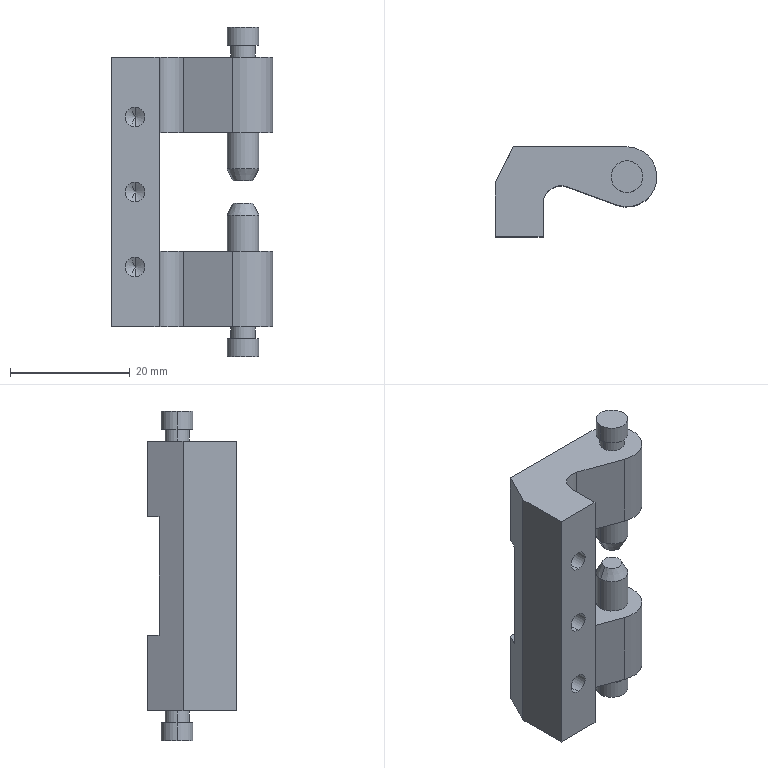Part | SolidWorks | features BaseBody 1 | 1 solid | 51 faces | box 27 x 15 x 55 mm | volume 8868 mm3 | cylinder 22 | plane 19 | cone 10 | commonest cylinder face diameters 5.3 x8 3.3 x6 4.101 x4 6 x2 10 x2
STEP:
#1=CARTESIAN_POINT('',(4.,13.,-9.85));
#2=VERTEX_POINT('',#1);
#3=CARTESIAN_POINT('',(-2.,13.,-9.85));
#4=VERTEX_POINT('',#3);
#5=CARTESIAN_POINT('',(11.,13.,-9.85));
#6=DIRECTION('',(-1.,0.,0.));
#7=VECTOR('',#6,1000.);
#8=LINE('',#5,#7);
#9=EDGE_CURVE('',#2,#4,#8,.T.);
#10=ORIENTED_EDGE('',*,*,#9,.T.);
#11=CARTESIAN_POINT('',(-2.,13.,9.85));
#12=VERTEX_POINT('',#11);
#13=CARTESIAN_POINT('',(-2.,13.,22.5));
#14=DIRECTION('',(0.,0.,-1.));
#15=VECTOR('',#14,1000.);
#16=LINE('',#13,#15);
#17=EDGE_CURVE('',#12,#4,#16,.T.);
#18=ORIENTED_EDGE('',*,*,#17,.F.);
#19=CARTESIAN_POINT('',(4.,13.,9.85));
#20=VERTEX_POINT('',#19);
#21=CARTESIAN_POINT('',(11.,13.,9.85));
#22=DIRECTION('',(-1.,0.,0.));
#23=VECTOR('',#22,1000.);
#24=LINE('',#21,#23);
#25=EDGE_CURVE('',#20,#12,#24,.T.);
#26=ORIENTED_EDGE('',*,*,#25,.F.);
#27=CARTESIAN_POINT('',(4.,13.,22.5));
#28=DIRECTION('',(0.,0.,1.));
#29=VECTOR('',#28,1000.);
#30=LINE('',#27,#29);
#31=EDGE_CURVE('',#2,#20,#30,.T.);
#32=ORIENTED_EDGE('',*,*,#31,.F.);
#33=EDGE_LOOP('',(#10,#18,#26,#32));
#34=FACE_OUTER_BOUND('',#33,.T.);
#35=CARTESIAN_POINT('',(11.,13.,-9.85));
#36=DIRECTION('',(0.,-1.,0.));
#37=DIRECTION('',(0.,0.,-1.));
#38=AXIS2_PLACEMENT_3D('',#35,#36,#37);
#39=PLANE('',#38);
#40=ADVANCED_FACE('',(#34),#39,.F.);
#41=CARTESIAN_POINT('',(0.,10.1,1.65));
#42=VERTEX_POINT('',#41);
#43=CARTESIAN_POINT('',(0.,0.,1.65));
#44=VERTEX_POINT('',#43);
#45=CARTESIAN_POINT('',(0.,0.,1.65));
#46=DIRECTION('',(0.,-1.,0.));
#47=VECTOR('',#46,1000.);
#48=LINE('',#45,#47);
#49=EDGE_CURVE('',#42,#44,#48,.T.);
#50=ORIENTED_EDGE('',*,*,#49,.F.);
#51=CARTESIAN_POINT('',(0.,10.1,-1.65));
#52=VERTEX_POINT('',#51);
#53=CARTESIAN_POINT('',(0.,10.1,0.));
#54=DIRECTION('',(0.,-1.,0.));
#55=DIRECTION('',(0.,0.,-1.));
#56=AXIS2_PLACEMENT_3D('',#53,#54,#55);
#57=CIRCLE('',#56,1.65);
#58=EDGE_CURVE('',#52,#42,#57,.T.);
#59=ORIENTED_EDGE('',*,*,#58,.F.);
#60=CARTESIAN_POINT('',(0.,0.,-1.65));
#61=VERTEX_POINT('',#60);
#62=CARTESIAN_POINT('',(0.,0.,-1.65));
#63=DIRECTION('',(0.,-1.,0.));
#64=VECTOR('',#63,1000.);
#65=LINE('',#62,#64);
#66=EDGE_CURVE('',#52,#61,#65,.T.);
#67=ORIENTED_EDGE('',*,*,#66,.T.);
#68=CARTESIAN_POINT('',(0.,0.,0.));
#69=DIRECTION('',(0.,-1.,0.));
#70=DIRECTION('',(0.,0.,-1.));
#71=AXIS2_PLACEMENT_3D('',#68,#69,#70);
#72=CIRCLE('',#71,1.65);
#73=EDGE_CURVE('',#61,#44,#72,.T.);
#74=ORIENTED_EDGE('',*,*,#73,.T.);
#75=EDGE_LOOP('',(#50,#59,#67,#74));
#76=FACE_OUTER_BOUND('',#75,.T.);
#77=CARTESIAN_POINT('',(0.,0.,0.));
#78=DIRECTION('',(0.,-1.,0.));
#79=DIRECTION('',(0.,0.,-1.));
#80=AXIS2_PLACEMENT_3D('',#77,#78,#79);
#81=CYLINDRICAL_SURFACE('',#80,1.65);
#82=ADVANCED_FACE('',(#76),#81,.F.);
#83=CARTESIAN_POINT('',(0.,11.091,0.));
#84=VERTEX_POINT('',#83);
#85=CARTESIAN_POINT('',(0.,10.1,1.65));
#86=DIRECTION('',(0.,-0.515,0.8572));
#87=VECTOR('',#86,1000.);
#88=LINE('',#85,#87);
#89=EDGE_CURVE('',#84,#42,#88,.T.);
#90=ORIENTED_EDGE('',*,*,#89,.F.);
#91=CARTESIAN_POINT('',(0.,10.1,-1.65));
#92=DIRECTION('',(0.,-0.515,-0.8572));
#93=VECTOR('',#92,1000.);
#94=LINE('',#91,#93);
#95=EDGE_CURVE('',#84,#52,#94,.T.);
#96=ORIENTED_EDGE('',*,*,#95,.T.);
#97=ORIENTED_EDGE('',*,*,#58,.T.);
#98=EDGE_LOOP('',(#90,#96,#97));
#99=FACE_OUTER_BOUND('',#98,.T.);
#100=CARTESIAN_POINT('',(0.,10.1,0.));
#101=DIRECTION('',(0.,-1.,0.));
#102=DIRECTION('',(0.,0.,-1.));
#103=AXIS2_PLACEMENT_3D('',#100,#101,#102);
#104=CONICAL_SURFACE('',#103,1.65,1.03);
#105=ADVANCED_FACE('',(#99),#104,.F.);
#106=CARTESIAN_POINT('',(0.,10.1,14.15));
#107=VERTEX_POINT('',#106);
#108=CARTESIAN_POINT('',(0.,0.,14.15));
#109=VERTEX_POINT('',#108);
#110=CARTESIAN_POINT('',(0.,0.,14.15));
#111=DIRECTION('',(0.,-1.,0.));
#112=VECTOR('',#111,1000.);
#113=LINE('',#110,#112);
#114=EDGE_CURVE('',#107,#109,#113,.T.);
#115=ORIENTED_EDGE('',*,*,#114,.F.);
#116=CARTESIAN_POINT('',(0.,10.1,10.85));
#117=VERTEX_POINT('',#116);
#118=CARTESIAN_POINT('',(0.,10.1,12.5));
#119=DIRECTION('',(0.,-1.,0.));
#120=DIRECTION('',(0.,0.,-1.));
#121=AXIS2_PLACEMENT_3D('',#118,#119,#120);
#122=CIRCLE('',#121,1.65);
#123=EDGE_CURVE('',#117,#107,#122,.T.);
#124=ORIENTED_EDGE('',*,*,#123,.F.);
#125=CARTESIAN_POINT('',(0.,0.,10.85));
#126=VERTEX_POINT('',#125);
#127=CARTESIAN_POINT('',(0.,0.,10.85));
#128=DIRECTION('',(0.,-1.,0.));
#129=VECTOR('',#128,1000.);
#130=LINE('',#127,#129);
#131=EDGE_CURVE('',#117,#126,#130,.T.);
#132=ORIENTED_EDGE('',*,*,#131,.T.);
#133=CARTESIAN_POINT('',(0.,0.,12.5));
#134=DIRECTION('',(0.,-1.,0.));
#135=DIRECTION('',(0.,0.,-1.));
#136=AXIS2_PLACEMENT_3D('',#133,#134,#135);
#137=CIRCLE('',#136,1.65);
#138=EDGE_CURVE('',#126,#109,#137,.T.);
#139=ORIENTED_EDGE('',*,*,#138,.T.);
#140=EDGE_LOOP('',(#115,#124,#132,#139));
#141=FACE_OUTER_BOUND('',#140,.T.);
#142=CARTESIAN_POINT('',(0.,0.,12.5));
#143=DIRECTION('',(0.,-1.,0.));
#144=DIRECTION('',(0.,0.,-1.));
#145=AXIS2_PLACEMENT_3D('',#142,#143,#144);
#146=CYLINDRICAL_SURFACE('',#145,1.65);
#147=ADVANCED_FACE('',(#141),#146,.F.);
#148=CARTESIAN_POINT('',(0.,11.091,12.5));
#149=VERTEX_POINT('',#148);
#150=CARTESIAN_POINT('',(0.,10.1,14.15));
#151=DIRECTION('',(0.,-0.515,0.8572));
#152=VECTOR('',#151,1000.);
#153=LINE('',#150,#152);
#154=EDGE_CURVE('',#149,#107,#153,.T.);
#155=ORIENTED_EDGE('',*,*,#154,.F.);
#156=CARTESIAN_POINT('',(0.,10.1,10.85));
#157=DIRECTION('',(0.,-0.515,-0.8572));
#158=VECTOR('',#157,1000.);
#159=LINE('',#156,#158);
#160=EDGE_CURVE('',#149,#117,#159,.T.);
#161=ORIENTED_EDGE('',*,*,#160,.T.);
#162=ORIENTED_EDGE('',*,*,#123,.T.);
#163=EDGE_LOOP('',(#155,#161,#162));
#164=FACE_OUTER_BOUND('',#163,.T.);
#165=CARTESIAN_POINT('',(0.,10.1,12.5));
#166=DIRECTION('',(0.,-1.,0.));
#167=DIRECTION('',(0.,0.,-1.));
#168=AXIS2_PLACEMENT_3D('',#165,#166,#167);
#169=CONICAL_SURFACE('',#168,1.65,1.03);
#170=ADVANCED_FACE('',(#164),#169,.F.);
#171=CARTESIAN_POINT('',(0.,10.1,-10.85));
#172=VERTEX_POINT('',#171);
#173=CARTESIAN_POINT('',(0.,0.,-10.85));
#174=VERTEX_POINT('',#173);
#175=CARTESIAN_POINT('',(0.,0.,-10.85));
#176=DIRECTION('',(0.,-1.,0.));
#177=VECTOR('',#176,1000.);
#178=LINE('',#175,#177);
#179=EDGE_CURVE('',#172,#174,#178,.T.);
#180=ORIENTED_EDGE('',*,*,#179,.F.);
#181=CARTESIAN_POINT('',(0.,10.1,-14.15));
#182=VERTEX_POINT('',#181);
#183=CARTESIAN_POINT('',(0.,10.1,-12.5));
#184=DIRECTION('',(0.,-1.,0.));
#185=DIRECTION('',(0.,0.,-1.));
#186=AXIS2_PLACEMENT_3D('',#183,#184,#185);
#187=CIRCLE('',#186,1.65);
#188=EDGE_CURVE('',#182,#172,#187,.T.);
#189=ORIENTED_EDGE('',*,*,#188,.F.);
#190=CARTESIAN_POINT('',(0.,0.,-14.15));
#191=VERTEX_POINT('',#190);
#192=CARTESIAN_POINT('',(0.,0.,-14.15));
#193=DIRECTION('',(0.,-1.,0.));
#194=VECTOR('',#193,1000.);
#195=LINE('',#192,#194);
#196=EDGE_CURVE('',#182,#191,#195,.T.);
#197=ORIENTED_EDGE('',*,*,#196,.T.);
#198=CARTESIAN_POINT('',(0.,0.,-12.5));
#199=DIRECTION('',(0.,-1.,0.));
#200=DIRECTION('',(0.,0.,-1.));
#201=AXIS2_PLACEMENT_3D('',#198,#199,#200);
#202=CIRCLE('',#201,1.65);
#203=EDGE_CURVE('',#191,#174,#202,.T.);
#204=ORIENTED_EDGE('',*,*,#203,.T.);
#205=EDGE_LOOP('',(#180,#189,#197,#204));
#206=FACE_OUTER_BOUND('',#205,.T.);
#207=CARTESIAN_POINT('',(0.,0.,-12.5));
#208=DIRECTION('',(0.,-1.,0.));
#209=DIRECTION('',(0.,0.,-1.));
#210=AXIS2_PLACEMENT_3D('',#207,#208,#209);
#211=CYLINDRICAL_SURFACE('',#210,1.65);
#212=ADVANCED_FACE('',(#206),#211,.F.);
#213=CARTESIAN_POINT('',(0.,11.091,-12.5));
#214=VERTEX_POINT('',#213);
#215=CARTESIAN_POINT('',(0.,10.1,-10.85));
#216=DIRECTION('',(0.,-0.515,0.8572));
#217=VECTOR('',#216,1000.);
#218=LINE('',#215,#217);
#219=EDGE_CURVE('',#214,#172,#218,.T.);
#220=ORIENTED_EDGE('',*,*,#219,.F.);
#221=CARTESIAN_POINT('',(0.,10.1,-14.15));
#222=DIRECTION('',(0.,-0.515,-0.8572));
#223=VECTOR('',#222,1000.);
#224=LINE('',#221,#223);
#225=EDGE_CURVE('',#214,#182,#224,.T.);
#226=ORIENTED_EDGE('',*,*,#225,.T.);
#227=ORIENTED_EDGE('',*,*,#188,.T.);
#228=EDGE_LOOP('',(#220,#226,#227));
#229=FACE_OUTER_BOUND('',#228,.T.);
#230=CARTESIAN_POINT('',(0.,10.1,-12.5));
#231=DIRECTION('',(0.,-1.,0.));
#232=DIRECTION('',(0.,0.,-1.));
#233=AXIS2_PLACEMENT_3D('',#230,#231,#232);
#234=CONICAL_SURFACE('',#233,1.65,1.03);
#235=ADVANCED_FACE('',(#229),#234,.F.);
#236=CARTESIAN_POINT('',(20.65,10.,27.5));
#237=VERTEX_POINT('',#236);
#238=CARTESIAN_POINT('',(20.65,10.,24.5));
#239=VERTEX_POINT('',#238);
#240=CARTESIAN_POINT('',(20.65,10.,27.5));
#241=DIRECTION('',(0.,0.,-1.));
#242=VECTOR('',#241,1000.);
#243=LINE('',#240,#242);
#244=EDGE_CURVE('',#237,#239,#243,.T.);
#245=ORIENTED_EDGE('',*,*,#244,.F.);
#246=CARTESIAN_POINT('',(15.35,10.,27.5));
#247=VERTEX_POINT('',#246);
#248=CARTESIAN_POINT('',(18.,10.,27.5));
#249=DIRECTION('',(0.,0.,-1.));
#250=DIRECTION('',(-1.,0.,0.));
#251=AXIS2_PLACEMENT_3D('',#248,#249,#250);
#252=CIRCLE('',#251,2.65);
#253=EDGE_CURVE('',#237,#247,#252,.T.);
#254=ORIENTED_EDGE('',*,*,#253,.T.);
#255=CARTESIAN_POINT('',(15.35,10.,24.5));
#256=VERTEX_POINT('',#255);
#257=CARTESIAN_POINT('',(15.35,10.,27.5));
#258=DIRECTION('',(0.,0.,-1.));
#259=VECTOR('',#258,1000.);
#260=LINE('',#257,#259);
#261=EDGE_CURVE('',#247,#256,#260,.T.);
#262=ORIENTED_EDGE('',*,*,#261,.T.);
#263=CARTESIAN_POINT('',(18.,10.,24.5));
#264=DIRECTION('',(0.,0.,-1.));
#265=DIRECTION('',(-1.,0.,0.));
#266=AXIS2_PLACEMENT_3D('',#263,#264,#265);
#267=CIRCLE('',#266,2.65);
#268=EDGE_CURVE('',#239,#256,#267,.T.);
#269=ORIENTED_EDGE('',*,*,#268,.F.);
#270=EDGE_LOOP('',(#245,#254,#262,#269));
#271=FACE_OUTER_BOUND('',#270,.T.);
#272=CARTESIAN_POINT('',(18.,10.,27.5));
#273=DIRECTION('',(0.,0.,-1.));
#274=DIRECTION('',(-1.,0.,0.));
#275=AXIS2_PLACEMENT_3D('',#272,#273,#274);
#276=CYLINDRICAL_SURFACE('',#275,2.65);
#277=ADVANCED_FACE('',(#271),#276,.T.);
#278=CARTESIAN_POINT('',(18.,10.,27.5));
#279=DIRECTION('',(0.,0.,-1.));
#280=DIRECTION('',(-1.,0.,0.));
#281=AXIS2_PLACEMENT_3D('',#278,#279,#280);
#282=CIRCLE('',#281,2.65);
#283=EDGE_CURVE('',#247,#237,#282,.T.);
#284=ORIENTED_EDGE('',*,*,#283,.F.);
#285=ORIENTED_EDGE('',*,*,#253,.F.);
#286=EDGE_LOOP('',(#284,#285));
#287=FACE_OUTER_BOUND('',#286,.T.);
#288=CARTESIAN_POINT('',(18.,10.,27.5));
#289=DIRECTION('',(0.,0.,1.));
#290=DIRECTION('',(1.,0.,0.));
#291=AXIS2_PLACEMENT_3D('',#288,#289,#290);
#292=PLANE('',#291);
#293=ADVANCED_FACE('',(#287),#292,.T.);
#294=CARTESIAN_POINT('',(20.05,10.,24.5));
#295=VERTEX_POINT('',#294);
#296=CARTESIAN_POINT('',(20.05,10.,22.5));
#297=VERTEX_POINT('',#296);
#298=CARTESIAN_POINT('',(20.05,10.,24.5));
#299=DIRECTION('',(0.,0.,-1.));
#300=VECTOR('',#299,1000.);
#301=LINE('',#298,#300);
#302=EDGE_CURVE('',#295,#297,#301,.T.);
#303=ORIENTED_EDGE('',*,*,#302,.F.);
#304=CARTESIAN_POINT('',(15.95,10.,24.5));
#305=VERTEX_POINT('',#304);
#306=CARTESIAN_POINT('',(18.,10.,24.5));
#307=DIRECTION('',(0.,0.,-1.));
#308=DIRECTION('',(-1.,0.,0.));
#309=AXIS2_PLACEMENT_3D('',#306,#307,#308);
#310=CIRCLE('',#309,2.05);
#311=EDGE_CURVE('',#295,#305,#310,.T.);
#312=ORIENTED_EDGE('',*,*,#311,.T.);
#313=CARTESIAN_POINT('',(15.95,10.,22.5));
#314=VERTEX_POINT('',#313);
#315=CARTESIAN_POINT('',(15.95,10.,24.5));
#316=DIRECTION('',(0.,0.,-1.));
#317=VECTOR('',#316,1000.);
#318=LINE('',#315,#317);
#319=EDGE_CURVE('',#305,#314,#318,.T.);
#320=ORIENTED_EDGE('',*,*,#319,.T.);
#321=CARTESIAN_POINT('',(18.,10.,22.5));
#322=DIRECTION('',(0.,0.,-1.));
#323=DIRECTION('',(-1.,0.,0.));
#324=AXIS2_PLACEMENT_3D('',#321,#322,#323);
#325=CIRCLE('',#324,2.05);
#326=EDGE_CURVE('',#297,#314,#325,.T.);
#327=ORIENTED_EDGE('',*,*,#326,.F.);
#328=EDGE_LOOP('',(#303,#312,#320,#327));
#329=FACE_OUTER_BOUND('',#328,.T.);
#330=CARTESIAN_POINT('',(18.,10.,24.5));
#331=DIRECTION('',(0.,0.,-1.));
#332=DIRECTION('',(-1.,0.,0.));
#333=AXIS2_PLACEMENT_3D('',#330,#331,#332);
#334=CYLINDRICAL_SURFACE('',#333,2.05);
#335=ADVANCED_FACE('',(#329),#334,.T.);
#336=CARTESIAN_POINT('',(18.,10.,24.5));
#337=DIRECTION('',(0.,0.,-1.));
#338=DIRECTION('',(-1.,0.,0.));
#339=AXIS2_PLACEMENT_3D('',#336,#337,#338);
#340=CIRCLE('',#339,2.05);
#341=EDGE_CURVE('',#305,#295,#340,.T.);
#342=ORIENTED_EDGE('',*,*,#341,.F.);
#343=ORIENTED_EDGE('',*,*,#311,.F.);
#344=EDGE_LOOP('',(#342,#343));
#345=FACE_BOUND('',#344,.T.);
#346=CARTESIAN_POINT('',(18.,10.,24.5));
#347=DIRECTION('',(0.,0.,-1.));
#348=DIRECTION('',(-1.,0.,0.));
#349=AXIS2_PLACEMENT_3D('',#346,#347,#348);
#350=CIRCLE('',#349,2.65);
#351=EDGE_CURVE('',#256,#239,#350,.T.);
#352=ORIENTED_EDGE('',*,*,#351,.T.);
#353=ORIENTED_EDGE('',*,*,#268,.T.);
#354=EDGE_LOOP('',(#352,#353));
#355=FACE_OUTER_BOUND('',#354,.T.);
#356=CARTESIAN_POINT('',(18.,10.,24.5));
#357=DIRECTION('',(0.,0.,1.));
#358=DIRECTION('',(1.,0.,0.));
#359=AXIS2_PLACEMENT_3D('',#356,#357,#358);
#360=PLANE('',#359);
#361=ADVANCED_FACE('',(#345,#355),#360,.F.);
#362=CARTESIAN_POINT('',(16.35,10.,1.85));
#363=VERTEX_POINT('',#362);
#364=CARTESIAN_POINT('',(15.35,10.,3.85));
#365=VERTEX_POINT('',#364);
#366=CARTESIAN_POINT('',(15.35,10.,3.85));
#367=DIRECTION('',(-0.4472,0.,0.8944));
#368=VECTOR('',#367,1000.);
#369=LINE('',#366,#368);
#370=EDGE_CURVE('',#363,#365,#369,.T.);
#371=ORIENTED_EDGE('',*,*,#370,.F.);
#372=CARTESIAN_POINT('',(19.65,10.,1.85));
#373=VERTEX_POINT('',#372);
#374=CARTESIAN_POINT('',(18.,10.,1.85));
#375=DIRECTION('',(0.,0.,-1.));
#376=DIRECTION('',(-1.,0.,0.));
#377=AXIS2_PLACEMENT_3D('',#374,#375,#376);
#378=CIRCLE('',#377,1.65);
#379=EDGE_CURVE('',#373,#363,#378,.T.);
#380=ORIENTED_EDGE('',*,*,#379,.F.);
#381=CARTESIAN_POINT('',(20.65,10.,3.85));
#382=VERTEX_POINT('',#381);
#383=CARTESIAN_POINT('',(20.65,10.,3.85));
#384=DIRECTION('',(0.4472,0.,0.8944));
#385=VECTOR('',#384,1000.);
#386=LINE('',#383,#385);
#387=EDGE_CURVE('',#373,#382,#386,.T.);
#388=ORIENTED_EDGE('',*,*,#387,.T.);
#389=CARTESIAN_POINT('',(18.,10.,3.85));
#390=DIRECTION('',(0.,0.,1.));
#391=DIRECTION('',(-1.,0.,0.));
#392=AXIS2_PLACEMENT_3D('',#389,#390,#391);
#393=CIRCLE('',#392,2.65);
#394=EDGE_CURVE('',#365,#382,#393,.T.);
#395=ORIENTED_EDGE('',*,*,#394,.F.);
#396=EDGE_LOOP('',(#371,#380,#388,#395));
#397=FACE_OUTER_BOUND('',#396,.T.);
#398=CARTESIAN_POINT('',(18.,10.,3.85));
#399=DIRECTION('',(0.,0.,1.));
#400=DIRECTION('',(1.,0.,0.));
#401=AXIS2_PLACEMENT_3D('',#398,#399,#400);
#402=CONICAL_SURFACE('',#401,2.65,0.4636);
#403=ADVANCED_FACE('',(#397),#402,.T.);
#404=ORIENTED_EDGE('',*,*,#379,.T.);
#405=CARTESIAN_POINT('',(18.,10.,1.85));
#406=DIRECTION('',(0.,0.,-1.));
#407=DIRECTION('',(-1.,0.,0.));
#408=AXIS2_PLACEMENT_3D('',#405,#406,#407);
#409=CIRCLE('',#408,1.65);
#410=EDGE_CURVE('',#363,#373,#409,.T.);
#411=ORIENTED_EDGE('',*,*,#410,.T.);
#412=EDGE_LOOP('',(#404,#411));
#413=FACE_OUTER_BOUND('',#412,.T.);
#414=CARTESIAN_POINT('',(18.,10.,1.85));
#415=DIRECTION('',(0.,0.,-1.));
#416=DIRECTION('',(0.,-1.,0.));
#417=AXIS2_PLACEMENT_3D('',#414,#415,#416);
#418=PLANE('',#417);
#419=ADVANCED_FACE('',(#413),#418,.T.);
#420=CARTESIAN_POINT('',(15.35,10.,9.85));
#421=VERTEX_POINT('',#420);
#422=CARTESIAN_POINT('',(15.35,10.,1.85));
#423=DIRECTION('',(0.,0.,1.));
#424=VECTOR('',#423,1000.);
#425=LINE('',#422,#424);
#426=EDGE_CURVE('',#365,#421,#425,.T.);
#427=ORIENTED_EDGE('',*,*,#426,.F.);
#428=ORIENTED_EDGE('',*,*,#394,.T.);
#429=CARTESIAN_POINT('',(20.65,10.,9.85));
#430=VERTEX_POINT('',#429);
#431=CARTESIAN_POINT('',(20.65,10.,1.85));
#432=DIRECTION('',(0.,0.,1.));
#433=VECTOR('',#432,1000.);
#434=LINE('',#431,#433);
#435=EDGE_CURVE('',#382,#430,#434,.T.);
#436=ORIENTED_EDGE('',*,*,#435,.T.);
#437=CARTESIAN_POINT('',(18.,10.,9.85));
#438=DIRECTION('',(0.,0.,1.));
#439=DIRECTION('',(1.,0.,0.));
#440=AXIS2_PLACEMENT_3D('',#437,#438,#439);
#441=CIRCLE('',#440,2.65);
#442=EDGE_CURVE('',#421,#430,#441,.T.);
#443=ORIENTED_EDGE('',*,*,#442,.F.);
#444=EDGE_LOOP('',(#427,#428,#436,#443));
#445=FACE_OUTER_BOUND('',#444,.T.);
#446=CARTESIAN_POINT('',(18.,10.,1.85));
#447=DIRECTION('',(0.,0.,1.));
#448=DIRECTION('',(1.,0.,0.));
#449=AXIS2_PLACEMENT_3D('',#446,#447,#448);
#450=CYLINDRICAL_SURFACE('',#449,2.65);
#451=ADVANCED_FACE('',(#445),#450,.T.);
#452=CARTESIAN_POINT('',(15.35,10.,-27.5));
#453=VERTEX_POINT('',#452);
#454=CARTESIAN_POINT('',(15.35,10.,-24.5));
#455=VERTEX_POINT('',#454);
#456=CARTESIAN_POINT('',(15.35,10.,-27.5));
#457=DIRECTION('',(0.,0.,1.));
#458=VECTOR('',#457,1000.);
#459=LINE('',#456,#458);
#460=EDGE_CURVE('',#453,#455,#459,.T.);
#461=ORIENTED_EDGE('',*,*,#460,.F.);
#462=CARTESIAN_POINT('',(20.65,10.,-27.5));
#463=VERTEX_POINT('',#462);
#464=CARTESIAN_POINT('',(18.,10.,-27.5));
#465=DIRECTION('',(0.,0.,-1.));
#466=DIRECTION('',(-1.,0.,0.));
#467=AXIS2_PLACEMENT_3D('',#464,#465,#466);
#468=CIRCLE('',#467,2.65);
#469=EDGE_CURVE('',#463,#453,#468,.T.);
#470=ORIENTED_EDGE('',*,*,#469,.F.);
#471=CARTESIAN_POINT('',(20.65,10.,-24.5));
#472=VERTEX_POINT('',#471);
#473=CARTESIAN_POINT('',(20.65,10.,-27.5));
#474=DIRECTION('',(0.,0.,1.));
#475=VECTOR('',#474,1000.);
#476=LINE('',#473,#475);
#477=EDGE_CURVE('',#463,#472,#476,.T.);
#478=ORIENTED_EDGE('',*,*,#477,.T.);
#479=CARTESIAN_POINT('',(18.,10.,-24.5));
#480=DIRECTION('',(0.,0.,-1.));
#481=DIRECTION('',(-1.,0.,0.));
#482=AXIS2_PLACEMENT_3D('',#479,#480,#481);
#483=CIRCLE('',#482,2.65);
#484=EDGE_CURVE('',#472,#455,#483,.T.);
#485=ORIENTED_EDGE('',*,*,#484,.T.);
#486=EDGE_LOOP('',(#461,#470,#478,#485));
#487=FACE_OUTER_BOUND('',#486,.T.);
#488=CARTESIAN_POINT('',(18.,10.,-27.5));
#489=DIRECTION('',(0.,0.,1.));
#490=DIRECTION('',(1.,0.,0.));
#491=AXIS2_PLACEMENT_3D('',#488,#489,#490);
#492=CYLINDRICAL_SURFACE('',#491,2.65);
#493=ADVANCED_FACE('',(#487),#492,.T.);
#494=ORIENTED_EDGE('',*,*,#469,.T.);
#495=CARTESIAN_POINT('',(18.,10.,-27.5));
#496=DIRECTION('',(0.,0.,-1.));
#497=DIRECTION('',(-1.,0.,0.));
#498=AXIS2_PLACEMENT_3D('',#495,#496,#497);
#499=CIRCLE('',#498,2.65);
#500=EDGE_CURVE('',#453,#463,#499,.T.);
#501=ORIENTED_EDGE('',*,*,#500,.T.);
#502=EDGE_LOOP('',(#494,#501));
#503=FACE_OUTER_BOUND('',#502,.T.);
#504=CARTESIAN_POINT('',(18.,10.,-27.5));
#505=DIRECTION('',(0.,0.,-1.));
#506=DIRECTION('',(0.,-1.,0.));
#507=AXIS2_PLACEMENT_3D('',#504,#505,#506);
#508=PLANE('',#507);
#509=ADVANCED_FACE('',(#503),#508,.T.);
#510=CARTESIAN_POINT('',(15.95,10.,-24.5));
#511=VERTEX_POINT('',#510);
#512=CARTESIAN_POINT('',(15.95,10.,-22.5));
#513=VERTEX_POINT('',#512);
#514=CARTESIAN_POINT('',(15.95,10.,-24.5));
#515=DIRECTION('',(0.,0.,1.));
#516=VECTOR('',#515,1000.);
#517=LINE('',#514,#516);
#518=EDGE_CURVE('',#511,#513,#517,.T.);
#519=ORIENTED_EDGE('',*,*,#518,.F.);
#520=CARTESIAN_POINT('',(20.05,10.,-24.5));
#521=VERTEX_POINT('',#520);
#522=CARTESIAN_POINT('',(18.,10.,-24.5));
#523=DIRECTION('',(0.,0.,-1.));
#524=DIRECTION('',(-1.,0.,0.));
#525=AXIS2_PLACEMENT_3D('',#522,#523,#524);
#526=CIRCLE('',#525,2.05);
#527=EDGE_CURVE('',#521,#511,#526,.T.);
#528=ORIENTED_EDGE('',*,*,#527,.F.);
#529=CARTESIAN_POINT('',(20.05,10.,-22.5));
#530=VERTEX_POINT('',#529);
#531=CARTESIAN_POINT('',(20.05,10.,-24.5));
#532=DIRECTION('',(0.,0.,1.));
#533=VECTOR('',#532,1000.);
#534=LINE('',#531,#533);
#535=EDGE_CURVE('',#521,#530,#534,.T.);
#536=ORIENTED_EDGE('',*,*,#535,.T.);
#537=CARTESIAN_POINT('',(18.,10.,-22.5));
#538=DIRECTION('',(0.,0.,-1.));
#539=DIRECTION('',(-1.,0.,0.));
#540=AXIS2_PLACEMENT_3D('',#537,#538,#539);
#541=CIRCLE('',#540,2.05);
#542=EDGE_CURVE('',#530,#513,#541,.T.);
#543=ORIENTED_EDGE('',*,*,#542,.T.);
#544=EDGE_LOOP('',(#519,#528,#536,#543));
#545=FACE_OUTER_BOUND('',#544,.T.);
#546=CARTESIAN_POINT('',(18.,10.,-24.5));
#547=DIRECTION('',(0.,0.,1.));
#548=DIRECTION('',(1.,0.,0.));
#549=AXIS2_PLACEMENT_3D('',#546,#547,#548);
#550=CYLINDRICAL_SURFACE('',#549,2.05);
#551=ADVANCED_FACE('',(#545),#550,.T.);
#552=ORIENTED_EDGE('',*,*,#527,.T.);
#553=CARTESIAN_POINT('',(18.,10.,-24.5));
#554=DIRECTION('',(0.,0.,-1.));
#555=DIRECTION('',(-1.,0.,0.));
#556=AXIS2_PLACEMENT_3D('',#553,#554,#555);
#557=CIRCLE('',#556,2.05);
#558=EDGE_CURVE('',#511,#521,#557,.T.);
#559=ORIENTED_EDGE('',*,*,#558,.T.);
#560=EDGE_LOOP('',(#552,#559));
#561=FACE_BOUND('',#560,.T.);
#562=ORIENTED_EDGE('',*,*,#484,.F.);
#563=CARTESIAN_POINT('',(18.,10.,-24.5));
#564=DIRECTION('',(0.,0.,-1.));
#565=DIRECTION('',(-1.,0.,0.));
#566=AXIS2_PLACEMENT_3D('',#563,#564,#565);
#567=CIRCLE('',#566,2.65);
#568=EDGE_CURVE('',#455,#472,#567,.T.);
#569=ORIENTED_EDGE('',*,*,#568,.F.);
#570=EDGE_LOOP('',(#562,#569));
#571=FACE_OUTER_BOUND('',#570,.T.);
#572=CARTESIAN_POINT('',(18.,10.,-24.5));
#573=DIRECTION('',(0.,0.,-1.));
#574=DIRECTION('',(0.,-1.,0.));
#575=AXIS2_PLACEMENT_3D('',#572,#573,#574);
#576=PLANE('',#575);
#577=ADVANCED_FACE('',(#561,#571),#576,.F.);
#578=CARTESIAN_POINT('',(19.65,10.,-1.85));
#579=VERTEX_POINT('',#578);
#580=CARTESIAN_POINT('',(20.65,10.,-3.85));
#581=VERTEX_POINT('',#580);
#582=CARTESIAN_POINT('',(19.65,10.,-1.85));
#583=DIRECTION('',(0.4472,0.,-0.8944));
#584=VECTOR('',#583,1000.);
#585=LINE('',#582,#584);
#586=EDGE_CURVE('',#579,#581,#585,.T.);
#587=ORIENTED_EDGE('',*,*,#586,.F.);
#588=CARTESIAN_POINT('',(16.35,10.,-1.85));
#589=VERTEX_POINT('',#588);
#590=CARTESIAN_POINT('',(18.,10.,-1.85));
#591=DIRECTION('',(0.,0.,1.));
#592=DIRECTION('',(1.,0.,0.));
#593=AXIS2_PLACEMENT_3D('',#590,#591,#592);
#594=CIRCLE('',#593,1.65);
#595=EDGE_CURVE('',#589,#579,#594,.T.);
#596=ORIENTED_EDGE('',*,*,#595,.F.);
#597=CARTESIAN_POINT('',(15.35,10.,-3.85));
#598=VERTEX_POINT('',#597);
#599=CARTESIAN_POINT('',(16.35,10.,-1.85));
#600=DIRECTION('',(-0.4472,0.,-0.8944));
#601=VECTOR('',#600,1000.);
#602=LINE('',#599,#601);
#603=EDGE_CURVE('',#589,#598,#602,.T.);
#604=ORIENTED_EDGE('',*,*,#603,.T.);
#605=CARTESIAN_POINT('',(18.,10.,-3.85));
#606=DIRECTION('',(0.,0.,-1.));
#607=DIRECTION('',(1.,0.,0.));
#608=AXIS2_PLACEMENT_3D('',#605,#606,#607);
#609=CIRCLE('',#608,2.65);
#610=EDGE_CURVE('',#581,#598,#609,.T.);
#611=ORIENTED_EDGE('',*,*,#610,.F.);
#612=EDGE_LOOP('',(#587,#596,#604,#611));
#613=FACE_OUTER_BOUND('',#612,.T.);
#614=CARTESIAN_POINT('',(18.,10.,-1.85));
#615=DIRECTION('',(0.,0.,-1.));
#616=DIRECTION('',(-1.,0.,0.));
#617=AXIS2_PLACEMENT_3D('',#614,#615,#616);
#618=CONICAL_SURFACE('',#617,1.65,0.4636);
#619=ADVANCED_FACE('',(#613),#618,.T.);
#620=ORIENTED_EDGE('',*,*,#595,.T.);
#621=CARTESIAN_POINT('',(18.,10.,-1.85));
#622=DIRECTION('',(0.,0.,1.));
#623=DIRECTION('',(1.,0.,0.));
#624=AXIS2_PLACEMENT_3D('',#621,#622,#623);
#625=CIRCLE('',#624,1.65);
#626=EDGE_CURVE('',#579,#589,#625,.T.);
#627=ORIENTED_EDGE('',*,*,#626,.T.);
#628=EDGE_LOOP('',(#620,#627));
#629=FACE_OUTER_BOUND('',#628,.T.);
#630=CARTESIAN_POINT('',(18.,10.,-1.85));
#631=DIRECTION('',(0.,0.,1.));
#632=DIRECTION('',(1.,0.,0.));
#633=AXIS2_PLACEMENT_3D('',#630,#631,#632);
#634=PLANE('',#633);
#635=ADVANCED_FACE('',(#629),#634,.T.);
#636=CARTESIAN_POINT('',(20.65,10.,-9.85));
#637=VERTEX_POINT('',#636);
#638=CARTESIAN_POINT('',(20.65,10.,-1.85));
#639=DIRECTION('',(0.,0.,-1.));
#640=VECTOR('',#639,1000.);
#641=LINE('',#638,#640);
#642=EDGE_CURVE('',#581,#637,#641,.T.);
#643=ORIENTED_EDGE('',*,*,#642,.F.);
#644=ORIENTED_EDGE('',*,*,#610,.T.);
#645=CARTESIAN_POINT('',(15.35,10.,-9.85));
#646=VERTEX_POINT('',#645);
#647=CARTESIAN_POINT('',(15.35,10.,-1.85));
#648=DIRECTION('',(0.,0.,-1.));
#649=VECTOR('',#648,1000.);
#650=LINE('',#647,#649);
#651=EDGE_CURVE('',#598,#646,#650,.T.);
#652=ORIENTED_EDGE('',*,*,#651,.T.);
#653=CARTESIAN_POINT('',(18.,10.,-9.85));
#654=DIRECTION('',(0.,0.,1.));
#655=DIRECTION('',(-1.,0.,0.));
#656=AXIS2_PLACEMENT_3D('',#653,#654,#655);
#657=CIRCLE('',#656,2.65);
#658=EDGE_CURVE('',#646,#637,#657,.T.);
#659=ORIENTED_EDGE('',*,*,#658,.T.);
#660=EDGE_LOOP('',(#643,#644,#652,#659));
#661=FACE_OUTER_BOUND('',#660,.T.);
#662=CARTESIAN_POINT('',(18.,10.,-1.85));
#663=DIRECTION('',(0.,0.,-1.));
#664=DIRECTION('',(-1.,0.,0.));
#665=AXIS2_PLACEMENT_3D('',#662,#663,#664);
#666=CYLINDRICAL_SURFACE('',#665,2.65);
#667=ADVANCED_FACE('',(#661),#666,.T.);
#668=CARTESIAN_POINT('',(18.,10.,9.85));
#669=DIRECTION('',(0.,0.,1.));
#670=DIRECTION('',(1.,0.,0.));
#671=AXIS2_PLACEMENT_3D('',#668,#669,#670);
#672=CIRCLE('',#671,2.65);
#673=EDGE_CURVE('',#430,#421,#672,.T.);
#674=ORIENTED_EDGE('',*,*,#673,.T.);
#675=ORIENTED_EDGE('',*,*,#442,.T.);
#676=EDGE_LOOP('',(#674,#675));
#677=FACE_BOUND('',#676,.T.);
#678=CARTESIAN_POINT('',(4.,5.49,9.85));
#679=VERTEX_POINT('',#678);
#680=CARTESIAN_POINT('',(4.,-60.,9.85));
#681=DIRECTION('',(0.,1.,0.));
#682=VECTOR('',#681,1000.);
#683=LINE('',#680,#682);
#684=EDGE_CURVE('',#679,#20,#683,.T.);
#685=ORIENTED_EDGE('',*,*,#684,.T.);
#686=ORIENTED_EDGE('',*,*,#25,.T.);
#687=CARTESIAN_POINT('',(-1.,15.,9.85));
#688=VERTEX_POINT('',#687);
#689=CARTESIAN_POINT('',(-4.,9.,9.85));
#690=DIRECTION('',(-0.4472,-0.8944,0.));
#691=VECTOR('',#690,1000.);
#692=LINE('',#689,#691);
#693=EDGE_CURVE('',#688,#12,#692,.T.);
#694=ORIENTED_EDGE('',*,*,#693,.F.);
#695=CARTESIAN_POINT('',(18.,15.,9.85));
#696=VERTEX_POINT('',#695);
#697=CARTESIAN_POINT('',(4.,15.,9.85));
#698=DIRECTION('',(1.,0.,0.));
#699=VECTOR('',#698,1000.);
#700=LINE('',#697,#699);
#701=EDGE_CURVE('',#688,#696,#700,.T.);
#702=ORIENTED_EDGE('',*,*,#701,.T.);
#703=CARTESIAN_POINT('',(16.29,5.302,9.85));
#704=VERTEX_POINT('',#703);
#705=CARTESIAN_POINT('',(18.,10.,9.85));
#706=DIRECTION('',(0.,0.,1.));
#707=DIRECTION('',(1.,0.,0.));
#708=AXIS2_PLACEMENT_3D('',#705,#706,#707);
#709=CIRCLE('',#708,5.);
#710=EDGE_CURVE('',#704,#696,#709,.T.);
#711=ORIENTED_EDGE('',*,*,#710,.F.);
#712=CARTESIAN_POINT('',(8.026,8.309,9.85));
#713=VERTEX_POINT('',#712);
#714=CARTESIAN_POINT('',(16.29,5.302,9.85));
#715=DIRECTION('',(0.9397,-0.342,0.));
#716=VECTOR('',#715,1000.);
#717=LINE('',#714,#716);
#718=EDGE_CURVE('',#713,#704,#717,.T.);
#719=ORIENTED_EDGE('',*,*,#718,.F.);
#720=CARTESIAN_POINT('',(7.,5.49,9.85));
#721=DIRECTION('',(0.,0.,-1.));
#722=DIRECTION('',(1.,0.,0.));
#723=AXIS2_PLACEMENT_3D('',#720,#721,#722);
#724=CIRCLE('',#723,3.);
#725=EDGE_CURVE('',#679,#713,#724,.T.);
#726=ORIENTED_EDGE('',*,*,#725,.F.);
#727=EDGE_LOOP('',(#685,#686,#694,#702,#711,#719,#726));
#728=FACE_OUTER_BOUND('',#727,.T.);
#729=CARTESIAN_POINT('',(4.,-60.,9.85));
#730=DIRECTION('',(0.,0.,1.));
#731=DIRECTION('',(1.,0.,0.));
#732=AXIS2_PLACEMENT_3D('',#729,#730,#731);
#733=PLANE('',#732);
#734=ADVANCED_FACE('',(#677,#728),#733,.F.);
#735=ORIENTED_EDGE('',*,*,#658,.F.);
#736=CARTESIAN_POINT('',(18.,10.,-9.85));
#737=DIRECTION('',(0.,0.,1.));
#738=DIRECTION('',(-1.,0.,0.));
#739=AXIS2_PLACEMENT_3D('',#736,#737,#738);
#740=CIRCLE('',#739,2.65);
#741=EDGE_CURVE('',#637,#646,#740,.T.);
#742=ORIENTED_EDGE('',*,*,#741,.F.);
#743=EDGE_LOOP('',(#735,#742));
#744=FACE_BOUND('',#743,.T.);
#745=CARTESIAN_POINT('',(-1.,15.,-9.85));
#746=VERTEX_POINT('',#745);
#747=CARTESIAN_POINT('',(18.,15.,-9.85));
#748=VERTEX_POINT('',#747);
#749=CARTESIAN_POINT('',(-1.,15.,-9.85));
#750=DIRECTION('',(1.,0.,0.));
#751=VECTOR('',#750,1000.);
#752=LINE('',#749,#751);
#753=EDGE_CURVE('',#746,#748,#752,.T.);
#754=ORIENTED_EDGE('',*,*,#753,.F.);
#755=CARTESIAN_POINT('',(-4.,9.,-9.85));
#756=DIRECTION('',(0.4472,0.8944,0.));
#757=VECTOR('',#756,1000.);
#758=LINE('',#755,#757);
#759=EDGE_CURVE('',#4,#746,#758,.T.);
#760=ORIENTED_EDGE('',*,*,#759,.F.);
#761=ORIENTED_EDGE('',*,*,#9,.F.);
#762=CARTESIAN_POINT('',(4.,5.49,-9.85));
#763=VERTEX_POINT('',#762);
#764=CARTESIAN_POINT('',(4.,-60.,-9.85));
#765=DIRECTION('',(0.,1.,0.));
#766=VECTOR('',#765,1000.);
#767=LINE('',#764,#766);
#768=EDGE_CURVE('',#763,#2,#767,.T.);
#769=ORIENTED_EDGE('',*,*,#768,.F.);
#770=CARTESIAN_POINT('',(8.026,8.309,-9.85));
#771=VERTEX_POINT('',#770);
#772=CARTESIAN_POINT('',(7.,5.49,-9.85));
#773=DIRECTION('',(0.,0.,1.));
#774=DIRECTION('',(-1.,0.,0.));
#775=AXIS2_PLACEMENT_3D('',#772,#773,#774);
#776=CIRCLE('',#775,3.);
#777=EDGE_CURVE('',#771,#763,#776,.T.);
#778=ORIENTED_EDGE('',*,*,#777,.F.);
#779=CARTESIAN_POINT('',(16.29,5.302,-9.85));
#780=VERTEX_POINT('',#779);
#781=CARTESIAN_POINT('',(16.29,5.302,-9.85));
#782=DIRECTION('',(-0.9397,0.342,0.));
#783=VECTOR('',#782,1000.);
#784=LINE('',#781,#783);
#785=EDGE_CURVE('',#780,#771,#784,.T.);
#786=ORIENTED_EDGE('',*,*,#785,.F.);
#787=CARTESIAN_POINT('',(18.,10.,-9.85));
#788=DIRECTION('',(0.,0.,-1.));
#789=DIRECTION('',(-1.,0.,0.));
#790=AXIS2_PLACEMENT_3D('',#787,#788,#789);
#791=CIRCLE('',#790,5.);
#792=EDGE_CURVE('',#748,#780,#791,.T.);
#793=ORIENTED_EDGE('',*,*,#792,.F.);
#794=EDGE_LOOP('',(#754,#760,#761,#769,#778,#786,#793));
#795=FACE_OUTER_BOUND('',#794,.T.);
#796=CARTESIAN_POINT('',(4.,-60.,-9.85));
#797=DIRECTION('',(0.,0.,-1.));
#798=DIRECTION('',(0.,-1.,0.));
#799=AXIS2_PLACEMENT_3D('',#796,#797,#798);
#800=PLANE('',#799);
#801=ADVANCED_FACE('',(#744,#795),#800,.F.);
#802=ORIENTED_EDGE('',*,*,#542,.F.);
#803=CARTESIAN_POINT('',(18.,10.,-22.5));
#804=DIRECTION('',(0.,0.,-1.));
#805=DIRECTION('',(-1.,0.,0.));
#806=AXIS2_PLACEMENT_3D('',#803,#804,#805);
#807=CIRCLE('',#806,2.05);
#808=EDGE_CURVE('',#513,#530,#807,.T.);
#809=ORIENTED_EDGE('',*,*,#808,.F.);
#810=EDGE_LOOP('',(#802,#809));
#811=FACE_BOUND('',#810,.T.);
#812=CARTESIAN_POINT('',(-4.,9.,-22.5));
#813=VERTEX_POINT('',#812);
#814=CARTESIAN_POINT('',(-4.,0.,-22.5));
#815=VERTEX_POINT('',#814);
#816=CARTESIAN_POINT('',(-4.,0.,-22.5));
#817=DIRECTION('',(0.,-1.,0.));
#818=VECTOR('',#817,1000.);
#819=LINE('',#816,#818);
#820=EDGE_CURVE('',#813,#815,#819,.T.);
#821=ORIENTED_EDGE('',*,*,#820,.F.);
#822=CARTESIAN_POINT('',(-1.,15.,-22.5));
#823=VERTEX_POINT('',#822);
#824=CARTESIAN_POINT('',(-4.,9.,-22.5));
#825=DIRECTION('',(-0.4472,-0.8944,0.));
#826=VECTOR('',#825,1000.);
#827=LINE('',#824,#826);
#828=EDGE_CURVE('',#823,#813,#827,.T.);
#829=ORIENTED_EDGE('',*,*,#828,.F.);
#830=CARTESIAN_POINT('',(18.,15.,-22.5));
#831=VERTEX_POINT('',#830);
#832=CARTESIAN_POINT('',(-1.,15.,-22.5));
#833=DIRECTION('',(-1.,0.,0.));
#834=VECTOR('',#833,1000.);
#835=LINE('',#832,#834);
#836=EDGE_CURVE('',#831,#823,#835,.T.);
#837=ORIENTED_EDGE('',*,*,#836,.F.);
#838=CARTESIAN_POINT('',(16.29,5.302,-22.5));
#839=VERTEX_POINT('',#838);
#840=CARTESIAN_POINT('',(18.,10.,-22.5));
#841=DIRECTION('',(0.,0.,1.));
#842=DIRECTION('',(1.,0.,0.));
#843=AXIS2_PLACEMENT_3D('',#840,#841,#842);
#844=CIRCLE('',#843,5.);
#845=EDGE_CURVE('',#839,#831,#844,.T.);
#846=ORIENTED_EDGE('',*,*,#845,.F.);
#847=CARTESIAN_POINT('',(8.026,8.309,-22.5));
#848=VERTEX_POINT('',#847);
#849=CARTESIAN_POINT('',(16.29,5.302,-22.5));
#850=DIRECTION('',(0.9397,-0.342,0.));
#851=VECTOR('',#850,1000.);
#852=LINE('',#849,#851);
#853=EDGE_CURVE('',#848,#839,#852,.T.);
#854=ORIENTED_EDGE('',*,*,#853,.F.);
#855=CARTESIAN_POINT('',(4.,5.49,-22.5));
#856=VERTEX_POINT('',#855);
#857=CARTESIAN_POINT('',(7.,5.49,-22.5));
#858=DIRECTION('',(0.,0.,-1.));
#859=DIRECTION('',(-1.,0.,0.));
#860=AXIS2_PLACEMENT_3D('',#857,#858,#859);
#861=CIRCLE('',#860,3.);
#862=EDGE_CURVE('',#856,#848,#861,.T.);
#863=ORIENTED_EDGE('',*,*,#862,.F.);
#864=CARTESIAN_POINT('',(4.,0.,-22.5));
#865=VERTEX_POINT('',#864);
#866=CARTESIAN_POINT('',(4.,5.49,-22.5));
#867=DIRECTION('',(0.,1.,0.));
#868=VECTOR('',#867,1000.);
#869=LINE('',#866,#868);
#870=EDGE_CURVE('',#865,#856,#869,.T.);
#871=ORIENTED_EDGE('',*,*,#870,.F.);
#872=CARTESIAN_POINT('',(-4.,0.,-22.5));
#873=DIRECTION('',(1.,0.,0.));
#874=VECTOR('',#873,1000.);
#875=LINE('',#872,#874);
#876=EDGE_CURVE('',#815,#865,#875,.T.);
#877=ORIENTED_EDGE('',*,*,#876,.F.);
#878=EDGE_LOOP('',(#821,#829,#837,#846,#854,#863,#871,#877));
#879=FACE_OUTER_BOUND('',#878,.T.);
#880=CARTESIAN_POINT('',(18.,10.,-22.5));
#881=DIRECTION('',(0.,0.,1.));
#882=DIRECTION('',(1.,0.,0.));
#883=AXIS2_PLACEMENT_3D('',#880,#881,#882);
#884=PLANE('',#883);
#885=ADVANCED_FACE('',(#811,#879),#884,.F.);
#886=CARTESIAN_POINT('',(18.,10.,22.5));
#887=DIRECTION('',(0.,0.,-1.));
#888=DIRECTION('',(-1.,0.,0.));
#889=AXIS2_PLACEMENT_3D('',#886,#887,#888);
#890=CIRCLE('',#889,2.05);
#891=EDGE_CURVE('',#314,#297,#890,.T.);
#892=ORIENTED_EDGE('',*,*,#891,.T.);
#893=ORIENTED_EDGE('',*,*,#326,.T.);
#894=EDGE_LOOP('',(#892,#893));
#895=FACE_BOUND('',#894,.T.);
#896=CARTESIAN_POINT('',(-4.,9.,22.5));
#897=VERTEX_POINT('',#896);
#898=CARTESIAN_POINT('',(-4.,0.,22.5));
#899=VERTEX_POINT('',#898);
#900=CARTESIAN_POINT('',(-4.,0.,22.5));
#901=DIRECTION('',(0.,-1.,0.));
#902=VECTOR('',#901,1000.);
#903=LINE('',#900,#902);
#904=EDGE_CURVE('',#897,#899,#903,.T.);
#905=ORIENTED_EDGE('',*,*,#904,.T.);
#906=CARTESIAN_POINT('',(4.,0.,22.5));
#907=VERTEX_POINT('',#906);
#908=CARTESIAN_POINT('',(-4.,0.,22.5));
#909=DIRECTION('',(1.,0.,0.));
#910=VECTOR('',#909,1000.);
#911=LINE('',#908,#910);
#912=EDGE_CURVE('',#899,#907,#911,.T.);
#913=ORIENTED_EDGE('',*,*,#912,.T.);
#914=CARTESIAN_POINT('',(4.,5.49,22.5));
#915=VERTEX_POINT('',#914);
#916=CARTESIAN_POINT('',(4.,5.49,22.5));
#917=DIRECTION('',(0.,1.,0.));
#918=VECTOR('',#917,1000.);
#919=LINE('',#916,#918);
#920=EDGE_CURVE('',#907,#915,#919,.T.);
#921=ORIENTED_EDGE('',*,*,#920,.T.);
#922=CARTESIAN_POINT('',(8.026,8.309,22.5));
#923=VERTEX_POINT('',#922);
#924=CARTESIAN_POINT('',(7.,5.49,22.5));
#925=DIRECTION('',(0.,0.,-1.));
#926=DIRECTION('',(-1.,0.,0.));
#927=AXIS2_PLACEMENT_3D('',#924,#925,#926);
#928=CIRCLE('',#927,3.);
#929=EDGE_CURVE('',#915,#923,#928,.T.);
#930=ORIENTED_EDGE('',*,*,#929,.T.);
#931=CARTESIAN_POINT('',(16.29,5.302,22.5));
#932=VERTEX_POINT('',#931);
#933=CARTESIAN_POINT('',(16.29,5.302,22.5));
#934=DIRECTION('',(0.9397,-0.342,0.));
#935=VECTOR('',#934,1000.);
#936=LINE('',#933,#935);
#937=EDGE_CURVE('',#923,#932,#936,.T.);
#938=ORIENTED_EDGE('',*,*,#937,.T.);
#939=CARTESIAN_POINT('',(18.,15.,22.5));
#940=VERTEX_POINT('',#939);
#941=CARTESIAN_POINT('',(18.,10.,22.5));
#942=DIRECTION('',(0.,0.,1.));
#943=DIRECTION('',(1.,0.,0.));
#944=AXIS2_PLACEMENT_3D('',#941,#942,#943);
#945=CIRCLE('',#944,5.);
#946=EDGE_CURVE('',#932,#940,#945,.T.);
#947=ORIENTED_EDGE('',*,*,#946,.T.);
#948=CARTESIAN_POINT('',(-1.,15.,22.5));
#949=VERTEX_POINT('',#948);
#950=CARTESIAN_POINT('',(-1.,15.,22.5));
#951=DIRECTION('',(-1.,0.,0.));
#952=VECTOR('',#951,1000.);
#953=LINE('',#950,#952);
#954=EDGE_CURVE('',#940,#949,#953,.T.);
#955=ORIENTED_EDGE('',*,*,#954,.T.);
#956=CARTESIAN_POINT('',(-4.,9.,22.5));
#957=DIRECTION('',(-0.4472,-0.8944,0.));
#958=VECTOR('',#957,1000.);
#959=LINE('',#956,#958);
#960=EDGE_CURVE('',#949,#897,#959,.T.);
#961=ORIENTED_EDGE('',*,*,#960,.T.);
#962=EDGE_LOOP('',(#905,#913,#921,#930,#938,#947,#955,#961));
#963=FACE_OUTER_BOUND('',#962,.T.);
#964=CARTESIAN_POINT('',(18.,10.,22.5));
#965=DIRECTION('',(0.,0.,1.));
#966=DIRECTION('',(1.,0.,0.));
#967=AXIS2_PLACEMENT_3D('',#964,#965,#966);
#968=PLANE('',#967);
#969=ADVANCED_FACE('',(#895,#963),#968,.T.);
#970=ORIENTED_EDGE('',*,*,#17,.T.);
#971=ORIENTED_EDGE('',*,*,#759,.T.);
#972=CARTESIAN_POINT('',(-1.,15.,22.5));
#973=DIRECTION('',(0.,0.,-1.));
#974=VECTOR('',#973,1000.);
#975=LINE('',#972,#974);
#976=EDGE_CURVE('',#746,#823,#975,.T.);
#977=ORIENTED_EDGE('',*,*,#976,.T.);
#978=ORIENTED_EDGE('',*,*,#828,.T.);
#979=CARTESIAN_POINT('',(-4.,9.,22.5));
#980=DIRECTION('',(0.,0.,-1.));
#981=VECTOR('',#980,1000.);
#982=LINE('',#979,#981);
#983=EDGE_CURVE('',#897,#813,#982,.T.);
#984=ORIENTED_EDGE('',*,*,#983,.F.);
#985=ORIENTED_EDGE('',*,*,#960,.F.);
#986=CARTESIAN_POINT('',(-1.,15.,22.5));
#987=DIRECTION('',(0.,0.,-1.));
#988=VECTOR('',#987,1000.);
#989=LINE('',#986,#988);
#990=EDGE_CURVE('',#949,#688,#989,.T.);
#991=ORIENTED_EDGE('',*,*,#990,.T.);
#992=ORIENTED_EDGE('',*,*,#693,.T.);
#993=EDGE_LOOP('',(#970,#971,#977,#978,#984,#985,#991,#992));
#994=FACE_OUTER_BOUND('',#993,.T.);
#995=CARTESIAN_POINT('',(-4.,9.,22.5));
#996=DIRECTION('',(0.8944,-0.4472,0.));
#997=DIRECTION('',(0.,0.,-1.));
#998=AXIS2_PLACEMENT_3D('',#995,#996,#997);
#999=PLANE('',#998);
#1000=ADVANCED_FACE('',(#994),#999,.F.);
#1001=ORIENTED_EDGE('',*,*,#701,.F.);
#1002=ORIENTED_EDGE('',*,*,#990,.F.);
#1003=ORIENTED_EDGE('',*,*,#954,.F.);
#1004=CARTESIAN_POINT('',(18.,15.,22.5));
#1005=DIRECTION('',(0.,0.,-1.));
#1006=VECTOR('',#1005,1000.);
#1007=LINE('',#1004,#1006);
#1008=EDGE_CURVE('',#940,#696,#1007,.T.);
#1009=ORIENTED_EDGE('',*,*,#1008,.T.);
#1010=EDGE_LOOP('',(#1001,#1002,#1003,#1009));
#1011=FACE_OUTER_BOUND('',#1010,.T.);
#1012=CARTESIAN_POINT('',(-1.,15.,22.5));
#1013=DIRECTION('',(0.,-1.,0.));
#1014=DIRECTION('',(0.,0.,-1.));
#1015=AXIS2_PLACEMENT_3D('',#1012,#1013,#1014);
#1016=PLANE('',#1015);
#1017=ADVANCED_FACE('',(#1011),#1016,.F.);
#1018=ORIENTED_EDGE('',*,*,#710,.T.);
#1019=ORIENTED_EDGE('',*,*,#1008,.F.);
#1020=ORIENTED_EDGE('',*,*,#946,.F.);
#1021=CARTESIAN_POINT('',(16.29,5.302,22.5));
#1022=DIRECTION('',(0.,0.,-1.));
#1023=VECTOR('',#1022,1000.);
#1024=LINE('',#1021,#1023);
#1025=EDGE_CURVE('',#932,#704,#1024,.T.);
#1026=ORIENTED_EDGE('',*,*,#1025,.T.);
#1027=EDGE_LOOP('',(#1018,#1019,#1020,#1026));
#1028=FACE_OUTER_BOUND('',#1027,.T.);
#1029=CARTESIAN_POINT('',(18.,10.,22.5));
#1030=DIRECTION('',(0.,0.,-1.));
#1031=DIRECTION('',(-1.,0.,0.));
#1032=AXIS2_PLACEMENT_3D('',#1029,#1030,#1031);
#1033=CYLINDRICAL_SURFACE('',#1032,5.);
#1034=ADVANCED_FACE('',(#1028),#1033,.T.);
#1035=CARTESIAN_POINT('',(8.026,8.309,22.5));
#1036=DIRECTION('',(0.,0.,-1.));
#1037=VECTOR('',#1036,1000.);
#1038=LINE('',#1035,#1037);
#1039=EDGE_CURVE('',#923,#713,#1038,.T.);
#1040=ORIENTED_EDGE('',*,*,#1039,.T.);
#1041=ORIENTED_EDGE('',*,*,#718,.T.);
#1042=ORIENTED_EDGE('',*,*,#1025,.F.);
#1043=ORIENTED_EDGE('',*,*,#937,.F.);
#1044=EDGE_LOOP('',(#1040,#1041,#1042,#1043));
#1045=FACE_OUTER_BOUND('',#1044,.T.);
#1046=CARTESIAN_POINT('',(16.29,5.302,22.5));
#1047=DIRECTION('',(0.342,0.9397,0.));
#1048=DIRECTION('',(0.,0.,-1.));
#1049=AXIS2_PLACEMENT_3D('',#1046,#1047,#1048);
#1050=PLANE('',#1049);
#1051=ADVANCED_FACE('',(#1045),#1050,.F.);
#1052=CARTESIAN_POINT('',(4.,5.49,22.5));
#1053=DIRECTION('',(0.,0.,-1.));
#1054=VECTOR('',#1053,1000.);
#1055=LINE('',#1052,#1054);
#1056=EDGE_CURVE('',#915,#679,#1055,.T.);
#1057=ORIENTED_EDGE('',*,*,#1056,.T.);
#1058=ORIENTED_EDGE('',*,*,#725,.T.);
#1059=ORIENTED_EDGE('',*,*,#1039,.F.);
#1060=ORIENTED_EDGE('',*,*,#929,.F.);
#1061=EDGE_LOOP('',(#1057,#1058,#1059,#1060));
#1062=FACE_OUTER_BOUND('',#1061,.T.);
#1063=CARTESIAN_POINT('',(7.,5.49,22.5));
#1064=DIRECTION('',(0.,0.,-1.));
#1065=DIRECTION('',(-1.,0.,0.));
#1066=AXIS2_PLACEMENT_3D('',#1063,#1064,#1065);
#1067=CYLINDRICAL_SURFACE('',#1066,3.);
#1068=ADVANCED_FACE('',(#1062),#1067,.F.);
#1069=ORIENTED_EDGE('',*,*,#768,.T.);
#1070=ORIENTED_EDGE('',*,*,#31,.T.);
#1071=ORIENTED_EDGE('',*,*,#684,.F.);
#1072=ORIENTED_EDGE('',*,*,#1056,.F.);
#1073=ORIENTED_EDGE('',*,*,#920,.F.);
#1074=CARTESIAN_POINT('',(4.,0.,22.5));
#1075=DIRECTION('',(0.,0.,-1.));
#1076=VECTOR('',#1075,1000.);
#1077=LINE('',#1074,#1076);
#1078=EDGE_CURVE('',#907,#865,#1077,.T.);
#1079=ORIENTED_EDGE('',*,*,#1078,.T.);
#1080=ORIENTED_EDGE('',*,*,#870,.T.);
#1081=CARTESIAN_POINT('',(4.,5.49,22.5));
#1082=DIRECTION('',(0.,0.,-1.));
#1083=VECTOR('',#1082,1000.);
#1084=LINE('',#1081,#1083);
#1085=EDGE_CURVE('',#763,#856,#1084,.T.);
#1086=ORIENTED_EDGE('',*,*,#1085,.F.);
#1087=EDGE_LOOP('',(#1069,#1070,#1071,#1072,#1073,#1079,#1080,#1086));
#1088=FACE_OUTER_BOUND('',#1087,.T.);
#1089=CARTESIAN_POINT('',(4.,5.49,22.5));
#1090=DIRECTION('',(-1.,0.,0.));
#1091=DIRECTION('',(0.,0.,1.));
#1092=AXIS2_PLACEMENT_3D('',#1089,#1090,#1091);
#1093=PLANE('',#1092);
#1094=ADVANCED_FACE('',(#1088),#1093,.F.);
#1095=ORIENTED_EDGE('',*,*,#203,.F.);
#1096=CARTESIAN_POINT('',(0.,0.,-12.5));
#1097=DIRECTION('',(0.,-1.,0.));
#1098=DIRECTION('',(0.,0.,-1.));
#1099=AXIS2_PLACEMENT_3D('',#1096,#1097,#1098);
#1100=CIRCLE('',#1099,1.65);
#1101=EDGE_CURVE('',#174,#191,#1100,.T.);
#1102=ORIENTED_EDGE('',*,*,#1101,.F.);
#1103=EDGE_LOOP('',(#1095,#1102));
#1104=FACE_BOUND('',#1103,.T.);
#1105=ORIENTED_EDGE('',*,*,#138,.F.);
#1106=CARTESIAN_POINT('',(0.,0.,12.5));
#1107=DIRECTION('',(0.,-1.,0.));
#1108=DIRECTION('',(0.,0.,-1.));
#1109=AXIS2_PLACEMENT_3D('',#1106,#1107,#1108);
#1110=CIRCLE('',#1109,1.65);
#1111=EDGE_CURVE('',#109,#126,#1110,.T.);
#1112=ORIENTED_EDGE('',*,*,#1111,.F.);
#1113=EDGE_LOOP('',(#1105,#1112));
#1114=FACE_BOUND('',#1113,.T.);
#1115=ORIENTED_EDGE('',*,*,#73,.F.);
#1116=CARTESIAN_POINT('',(0.,0.,0.));
#1117=DIRECTION('',(0.,-1.,0.));
#1118=DIRECTION('',(0.,0.,-1.));
#1119=AXIS2_PLACEMENT_3D('',#1116,#1117,#1118);
#1120=CIRCLE('',#1119,1.65);
#1121=EDGE_CURVE('',#44,#61,#1120,.T.);
#1122=ORIENTED_EDGE('',*,*,#1121,.F.);
#1123=EDGE_LOOP('',(#1115,#1122));
#1124=FACE_BOUND('',#1123,.T.);
#1125=ORIENTED_EDGE('',*,*,#876,.T.);
#1126=ORIENTED_EDGE('',*,*,#1078,.F.);
#1127=ORIENTED_EDGE('',*,*,#912,.F.);
#1128=CARTESIAN_POINT('',(-4.,0.,22.5));
#1129=DIRECTION('',(0.,0.,-1.));
#1130=VECTOR('',#1129,1000.);
#1131=LINE('',#1128,#1130);
#1132=EDGE_CURVE('',#899,#815,#1131,.T.);
#1133=ORIENTED_EDGE('',*,*,#1132,.T.);
#1134=EDGE_LOOP('',(#1125,#1126,#1127,#1133));
#1135=FACE_OUTER_BOUND('',#1134,.T.);
#1136=CARTESIAN_POINT('',(-4.,0.,22.5));
#1137=DIRECTION('',(0.,1.,0.));
#1138=DIRECTION('',(1.,0.,0.));
#1139=AXIS2_PLACEMENT_3D('',#1136,#1137,#1138);
#1140=PLANE('',#1139);
#1141=ADVANCED_FACE('',(#1104,#1114,#1124,#1135),#1140,.F.);
#1142=ORIENTED_EDGE('',*,*,#820,.T.);
#1143=ORIENTED_EDGE('',*,*,#1132,.F.);
#1144=ORIENTED_EDGE('',*,*,#904,.F.);
#1145=ORIENTED_EDGE('',*,*,#983,.T.);
#1146=EDGE_LOOP('',(#1142,#1143,#1144,#1145));
#1147=FACE_OUTER_BOUND('',#1146,.T.);
#1148=CARTESIAN_POINT('',(-4.,0.,22.5));
#1149=DIRECTION('',(1.,0.,0.));
#1150=DIRECTION('',(0.,1.,0.));
#1151=AXIS2_PLACEMENT_3D('',#1148,#1149,#1150);
#1152=PLANE('',#1151);
#1153=ADVANCED_FACE('',(#1147),#1152,.F.);
#1154=CARTESIAN_POINT('',(18.,15.,22.5));
#1155=DIRECTION('',(0.,0.,-1.));
#1156=VECTOR('',#1155,1000.);
#1157=LINE('',#1154,#1156);
#1158=EDGE_CURVE('',#748,#831,#1157,.T.);
#1159=ORIENTED_EDGE('',*,*,#1158,.F.);
#1160=ORIENTED_EDGE('',*,*,#792,.T.);
#1161=CARTESIAN_POINT('',(16.29,5.302,22.5));
#1162=DIRECTION('',(0.,0.,-1.));
#1163=VECTOR('',#1162,1000.);
#1164=LINE('',#1161,#1163);
#1165=EDGE_CURVE('',#780,#839,#1164,.T.);
#1166=ORIENTED_EDGE('',*,*,#1165,.T.);
#1167=ORIENTED_EDGE('',*,*,#845,.T.);
#1168=EDGE_LOOP('',(#1159,#1160,#1166,#1167));
#1169=FACE_OUTER_BOUND('',#1168,.T.);
#1170=CARTESIAN_POINT('',(18.,10.,22.5));
#1171=DIRECTION('',(0.,0.,-1.));
#1172=DIRECTION('',(-1.,0.,0.));
#1173=AXIS2_PLACEMENT_3D('',#1170,#1171,#1172);
#1174=CYLINDRICAL_SURFACE('',#1173,5.);
#1175=ADVANCED_FACE('',(#1169),#1174,.T.);
#1176=ORIENTED_EDGE('',*,*,#1165,.F.);
#1177=ORIENTED_EDGE('',*,*,#785,.T.);
#1178=CARTESIAN_POINT('',(8.026,8.309,22.5));
#1179=DIRECTION('',(0.,0.,-1.));
#1180=VECTOR('',#1179,1000.);
#1181=LINE('',#1178,#1180);
#1182=EDGE_CURVE('',#771,#848,#1181,.T.);
#1183=ORIENTED_EDGE('',*,*,#1182,.T.);
#1184=ORIENTED_EDGE('',*,*,#853,.T.);
#1185=EDGE_LOOP('',(#1176,#1177,#1183,#1184));
#1186=FACE_OUTER_BOUND('',#1185,.T.);
#1187=CARTESIAN_POINT('',(16.29,5.302,22.5));
#1188=DIRECTION('',(0.342,0.9397,0.));
#1189=DIRECTION('',(0.,0.,-1.));
#1190=AXIS2_PLACEMENT_3D('',#1187,#1188,#1189);
#1191=PLANE('',#1190);
#1192=ADVANCED_FACE('',(#1186),#1191,.F.);
#1193=ORIENTED_EDGE('',*,*,#1182,.F.);
#1194=ORIENTED_EDGE('',*,*,#777,.T.);
#1195=ORIENTED_EDGE('',*,*,#1085,.T.);
#1196=ORIENTED_EDGE('',*,*,#862,.T.);
#1197=EDGE_LOOP('',(#1193,#1194,#1195,#1196));
#1198=FACE_OUTER_BOUND('',#1197,.T.);
#1199=CARTESIAN_POINT('',(7.,5.49,22.5));
#1200=DIRECTION('',(0.,0.,-1.));
#1201=DIRECTION('',(-1.,0.,0.));
#1202=AXIS2_PLACEMENT_3D('',#1199,#1200,#1201);
#1203=CYLINDRICAL_SURFACE('',#1202,3.);
#1204=ADVANCED_FACE('',(#1198),#1203,.F.);
#1205=ORIENTED_EDGE('',*,*,#976,.F.);
#1206=ORIENTED_EDGE('',*,*,#753,.T.);
#1207=ORIENTED_EDGE('',*,*,#1158,.T.);
#1208=ORIENTED_EDGE('',*,*,#836,.T.);
#1209=EDGE_LOOP('',(#1205,#1206,#1207,#1208));
#1210=FACE_OUTER_BOUND('',#1209,.T.);
#1211=CARTESIAN_POINT('',(-1.,15.,22.5));
#1212=DIRECTION('',(0.,-1.,0.));
#1213=DIRECTION('',(0.,0.,-1.));
#1214=AXIS2_PLACEMENT_3D('',#1211,#1212,#1213);
#1215=PLANE('',#1214);
#1216=ADVANCED_FACE('',(#1210),#1215,.F.);
#1217=CARTESIAN_POINT('',(18.,10.,-3.85));
#1218=DIRECTION('',(0.,0.,-1.));
#1219=DIRECTION('',(1.,0.,0.));
#1220=AXIS2_PLACEMENT_3D('',#1217,#1218,#1219);
#1221=CIRCLE('',#1220,2.65);
#1222=EDGE_CURVE('',#598,#581,#1221,.T.);
#1223=ORIENTED_EDGE('',*,*,#1222,.T.);
#1224=ORIENTED_EDGE('',*,*,#642,.T.);
#1225=ORIENTED_EDGE('',*,*,#741,.T.);
#1226=ORIENTED_EDGE('',*,*,#651,.F.);
#1227=EDGE_LOOP('',(#1223,#1224,#1225,#1226));
#1228=FACE_OUTER_BOUND('',#1227,.T.);
#1229=CARTESIAN_POINT('',(18.,10.,-1.85));
#1230=DIRECTION('',(0.,0.,-1.));
#1231=DIRECTION('',(-1.,0.,0.));
#1232=AXIS2_PLACEMENT_3D('',#1229,#1230,#1231);
#1233=CYLINDRICAL_SURFACE('',#1232,2.65);
#1234=ADVANCED_FACE('',(#1228),#1233,.T.);
#1235=ORIENTED_EDGE('',*,*,#626,.F.);
#1236=ORIENTED_EDGE('',*,*,#586,.T.);
#1237=ORIENTED_EDGE('',*,*,#1222,.F.);
#1238=ORIENTED_EDGE('',*,*,#603,.F.);
#1239=EDGE_LOOP('',(#1235,#1236,#1237,#1238));
#1240=FACE_OUTER_BOUND('',#1239,.T.);
#1241=CARTESIAN_POINT('',(18.,10.,-1.85));
#1242=DIRECTION('',(0.,0.,-1.));
#1243=DIRECTION('',(-1.,0.,0.));
#1244=AXIS2_PLACEMENT_3D('',#1241,#1242,#1243);
#1245=CONICAL_SURFACE('',#1244,1.65,0.4636);
#1246=ADVANCED_FACE('',(#1240),#1245,.T.);
#1247=ORIENTED_EDGE('',*,*,#558,.F.);
#1248=ORIENTED_EDGE('',*,*,#518,.T.);
#1249=ORIENTED_EDGE('',*,*,#808,.T.);
#1250=ORIENTED_EDGE('',*,*,#535,.F.);
#1251=EDGE_LOOP('',(#1247,#1248,#1249,#1250));
#1252=FACE_OUTER_BOUND('',#1251,.T.);
#1253=CARTESIAN_POINT('',(18.,10.,-24.5));
#1254=DIRECTION('',(0.,0.,1.));
#1255=DIRECTION('',(1.,0.,0.));
#1256=AXIS2_PLACEMENT_3D('',#1253,#1254,#1255);
#1257=CYLINDRICAL_SURFACE('',#1256,2.05);
#1258=ADVANCED_FACE('',(#1252),#1257,.T.);
#1259=ORIENTED_EDGE('',*,*,#500,.F.);
#1260=ORIENTED_EDGE('',*,*,#460,.T.);
#1261=ORIENTED_EDGE('',*,*,#568,.T.);
#1262=ORIENTED_EDGE('',*,*,#477,.F.);
#1263=EDGE_LOOP('',(#1259,#1260,#1261,#1262));
#1264=FACE_OUTER_BOUND('',#1263,.T.);
#1265=CARTESIAN_POINT('',(18.,10.,-27.5));
#1266=DIRECTION('',(0.,0.,1.));
#1267=DIRECTION('',(1.,0.,0.));
#1268=AXIS2_PLACEMENT_3D('',#1265,#1266,#1267);
#1269=CYLINDRICAL_SURFACE('',#1268,2.65);
#1270=ADVANCED_FACE('',(#1264),#1269,.T.);
#1271=CARTESIAN_POINT('',(18.,10.,3.85));
#1272=DIRECTION('',(0.,0.,1.));
#1273=DIRECTION('',(-1.,0.,0.));
#1274=AXIS2_PLACEMENT_3D('',#1271,#1272,#1273);
#1275=CIRCLE('',#1274,2.65);
#1276=EDGE_CURVE('',#382,#365,#1275,.T.);
#1277=ORIENTED_EDGE('',*,*,#1276,.T.);
#1278=ORIENTED_EDGE('',*,*,#426,.T.);
#1279=ORIENTED_EDGE('',*,*,#673,.F.);
#1280=ORIENTED_EDGE('',*,*,#435,.F.);
#1281=EDGE_LOOP('',(#1277,#1278,#1279,#1280));
#1282=FACE_OUTER_BOUND('',#1281,.T.);
#1283=CARTESIAN_POINT('',(18.,10.,1.85));
#1284=DIRECTION('',(0.,0.,1.));
#1285=DIRECTION('',(1.,0.,0.));
#1286=AXIS2_PLACEMENT_3D('',#1283,#1284,#1285);
#1287=CYLINDRICAL_SURFACE('',#1286,2.65);
#1288=ADVANCED_FACE('',(#1282),#1287,.T.);
#1289=ORIENTED_EDGE('',*,*,#410,.F.);
#1290=ORIENTED_EDGE('',*,*,#370,.T.);
#1291=ORIENTED_EDGE('',*,*,#1276,.F.);
#1292=ORIENTED_EDGE('',*,*,#387,.F.);
#1293=EDGE_LOOP('',(#1289,#1290,#1291,#1292));
#1294=FACE_OUTER_BOUND('',#1293,.T.);
#1295=CARTESIAN_POINT('',(18.,10.,3.85));
#1296=DIRECTION('',(0.,0.,1.));
#1297=DIRECTION('',(1.,0.,0.));
#1298=AXIS2_PLACEMENT_3D('',#1295,#1296,#1297);
#1299=CONICAL_SURFACE('',#1298,2.65,0.4636);
#1300=ADVANCED_FACE('',(#1294),#1299,.T.);
#1301=ORIENTED_EDGE('',*,*,#341,.T.);
#1302=ORIENTED_EDGE('',*,*,#302,.T.);
#1303=ORIENTED_EDGE('',*,*,#891,.F.);
#1304=ORIENTED_EDGE('',*,*,#319,.F.);
#1305=EDGE_LOOP('',(#1301,#1302,#1303,#1304));
#1306=FACE_OUTER_BOUND('',#1305,.T.);
#1307=CARTESIAN_POINT('',(18.,10.,24.5));
#1308=DIRECTION('',(0.,0.,-1.));
#1309=DIRECTION('',(-1.,0.,0.));
#1310=AXIS2_PLACEMENT_3D('',#1307,#1308,#1309);
#1311=CYLINDRICAL_SURFACE('',#1310,2.05);
#1312=ADVANCED_FACE('',(#1306),#1311,.T.);
#1313=ORIENTED_EDGE('',*,*,#283,.T.);
#1314=ORIENTED_EDGE('',*,*,#244,.T.);
#1315=ORIENTED_EDGE('',*,*,#351,.F.);
#1316=ORIENTED_EDGE('',*,*,#261,.F.);
#1317=EDGE_LOOP('',(#1313,#1314,#1315,#1316));
#1318=FACE_OUTER_BOUND('',#1317,.T.);
#1319=CARTESIAN_POINT('',(18.,10.,27.5));
#1320=DIRECTION('',(0.,0.,-1.));
#1321=DIRECTION('',(-1.,0.,0.));
#1322=AXIS2_PLACEMENT_3D('',#1319,#1320,#1321);
#1323=CYLINDRICAL_SURFACE('',#1322,2.65);
#1324=ADVANCED_FACE('',(#1318),#1323,.T.);
#1325=ORIENTED_EDGE('',*,*,#225,.F.);
#1326=ORIENTED_EDGE('',*,*,#219,.T.);
#1327=CARTESIAN_POINT('',(0.,10.1,-12.5));
#1328=DIRECTION('',(0.,-1.,0.));
#1329=DIRECTION('',(0.,0.,-1.));
#1330=AXIS2_PLACEMENT_3D('',#1327,#1328,#1329);
#1331=CIRCLE('',#1330,1.65);
#1332=EDGE_CURVE('',#172,#182,#1331,.T.);
#1333=ORIENTED_EDGE('',*,*,#1332,.T.);
#1334=EDGE_LOOP('',(#1325,#1326,#1333));
#1335=FACE_OUTER_BOUND('',#1334,.T.);
#1336=CARTESIAN_POINT('',(0.,10.1,-12.5));
#1337=DIRECTION('',(0.,-1.,0.));
#1338=DIRECTION('',(0.,0.,-1.));
#1339=AXIS2_PLACEMENT_3D('',#1336,#1337,#1338);
#1340=CONICAL_SURFACE('',#1339,1.65,1.03);
#1341=ADVANCED_FACE('',(#1335),#1340,.F.);
#1342=ORIENTED_EDGE('',*,*,#1332,.F.);
#1343=ORIENTED_EDGE('',*,*,#179,.T.);
#1344=ORIENTED_EDGE('',*,*,#1101,.T.);
#1345=ORIENTED_EDGE('',*,*,#196,.F.);
#1346=EDGE_LOOP('',(#1342,#1343,#1344,#1345));
#1347=FACE_OUTER_BOUND('',#1346,.T.);
#1348=CARTESIAN_POINT('',(0.,0.,-12.5));
#1349=DIRECTION('',(0.,-1.,0.));
#1350=DIRECTION('',(0.,0.,-1.));
#1351=AXIS2_PLACEMENT_3D('',#1348,#1349,#1350);
#1352=CYLINDRICAL_SURFACE('',#1351,1.65);
#1353=ADVANCED_FACE('',(#1347),#1352,.F.);
#1354=ORIENTED_EDGE('',*,*,#160,.F.);
#1355=ORIENTED_EDGE('',*,*,#154,.T.);
#1356=CARTESIAN_POINT('',(0.,10.1,12.5));
#1357=DIRECTION('',(0.,-1.,0.));
#1358=DIRECTION('',(0.,0.,-1.));
#1359=AXIS2_PLACEMENT_3D('',#1356,#1357,#1358);
#1360=CIRCLE('',#1359,1.65);
#1361=EDGE_CURVE('',#107,#117,#1360,.T.);
#1362=ORIENTED_EDGE('',*,*,#1361,.T.);
#1363=EDGE_LOOP('',(#1354,#1355,#1362));
#1364=FACE_OUTER_BOUND('',#1363,.T.);
#1365=CARTESIAN_POINT('',(0.,10.1,12.5));
#1366=DIRECTION('',(0.,-1.,0.));
#1367=DIRECTION('',(0.,0.,-1.));
#1368=AXIS2_PLACEMENT_3D('',#1365,#1366,#1367);
#1369=CONICAL_SURFACE('',#1368,1.65,1.03);
#1370=ADVANCED_FACE('',(#1364),#1369,.F.);
#1371=ORIENTED_EDGE('',*,*,#1361,.F.);
#1372=ORIENTED_EDGE('',*,*,#114,.T.);
#1373=ORIENTED_EDGE('',*,*,#1111,.T.);
#1374=ORIENTED_EDGE('',*,*,#131,.F.);
#1375=EDGE_LOOP('',(#1371,#1372,#1373,#1374));
#1376=FACE_OUTER_BOUND('',#1375,.T.);
#1377=CARTESIAN_POINT('',(0.,0.,12.5));
#1378=DIRECTION('',(0.,-1.,0.));
#1379=DIRECTION('',(0.,0.,-1.));
#1380=AXIS2_PLACEMENT_3D('',#1377,#1378,#1379);
#1381=CYLINDRICAL_SURFACE('',#1380,1.65);
#1382=ADVANCED_FACE('',(#1376),#1381,.F.);
#1383=ORIENTED_EDGE('',*,*,#95,.F.);
#1384=ORIENTED_EDGE('',*,*,#89,.T.);
#1385=CARTESIAN_POINT('',(0.,10.1,0.));
#1386=DIRECTION('',(0.,-1.,0.));
#1387=DIRECTION('',(0.,0.,-1.));
#1388=AXIS2_PLACEMENT_3D('',#1385,#1386,#1387);
#1389=CIRCLE('',#1388,1.65);
#1390=EDGE_CURVE('',#42,#52,#1389,.T.);
#1391=ORIENTED_EDGE('',*,*,#1390,.T.);
#1392=EDGE_LOOP('',(#1383,#1384,#1391));
#1393=FACE_OUTER_BOUND('',#1392,.T.);
#1394=CARTESIAN_POINT('',(0.,10.1,0.));
#1395=DIRECTION('',(0.,-1.,0.));
#1396=DIRECTION('',(0.,0.,-1.));
#1397=AXIS2_PLACEMENT_3D('',#1394,#1395,#1396);
#1398=CONICAL_SURFACE('',#1397,1.65,1.03);
#1399=ADVANCED_FACE('',(#1393),#1398,.F.);
#1400=ORIENTED_EDGE('',*,*,#1390,.F.);
#1401=ORIENTED_EDGE('',*,*,#49,.T.);
#1402=ORIENTED_EDGE('',*,*,#1121,.T.);
#1403=ORIENTED_EDGE('',*,*,#66,.F.);
#1404=EDGE_LOOP('',(#1400,#1401,#1402,#1403));
#1405=FACE_OUTER_BOUND('',#1404,.T.);
#1406=CARTESIAN_POINT('',(0.,0.,0.));
#1407=DIRECTION('',(0.,-1.,0.));
#1408=DIRECTION('',(0.,0.,-1.));
#1409=AXIS2_PLACEMENT_3D('',#1406,#1407,#1408);
#1410=CYLINDRICAL_SURFACE('',#1409,1.65);
#1411=ADVANCED_FACE('',(#1405),#1410,.F.);
#1412=CLOSED_SHELL('',(#40,#82,#105,#147,#170,#212,#235,#277,#293,#335,#361,#403,#419,#451,#493,#509,#551,#577,#619,#635,#667,#734,#801,#885,#969,#1000,#1017,#1034,#1051,#1068,#1094,#1141,#1153,#1175,#1192,#1204,#1216,#1234,#1246,#1258,#1270,#1288,#1300,#1312,#1324,#1341,#1353,#1370,#1382,#1399,#1411));
#1413=MANIFOLD_SOLID_BREP('',#1412);
#1414=CARTESIAN_POINT('',(0.,0.,0.));
#1415=DIRECTION('',(0.,0.,1.));
#1416=DIRECTION('',(1.,0.,0.));
#1417=AXIS2_PLACEMENT_3D('',#1414,#1415,#1416);
#1418=(LENGTH_UNIT()NAMED_UNIT(*)SI_UNIT(.MILLI.,.METRE.));
#1419=UNCERTAINTY_MEASURE_WITH_UNIT(LENGTH_MEASURE(0.00001),#1418,'','');
#1420=(NAMED_UNIT(*)PLANE_ANGLE_UNIT()SI_UNIT($,.RADIAN.));
#1421=(NAMED_UNIT(*)SI_UNIT($,.STERADIAN.)SOLID_ANGLE_UNIT());
#1422=(GEOMETRIC_REPRESENTATION_CONTEXT(3)GLOBAL_UNCERTAINTY_ASSIGNED_CONTEXT((#1419))GLOBAL_UNIT_ASSIGNED_CONTEXT((#1418,#1420,#1421))REPRESENTATION_CONTEXT('',''));
#1423=ADVANCED_BREP_SHAPE_REPRESENTATION('',(#1413,#1417),#1422);